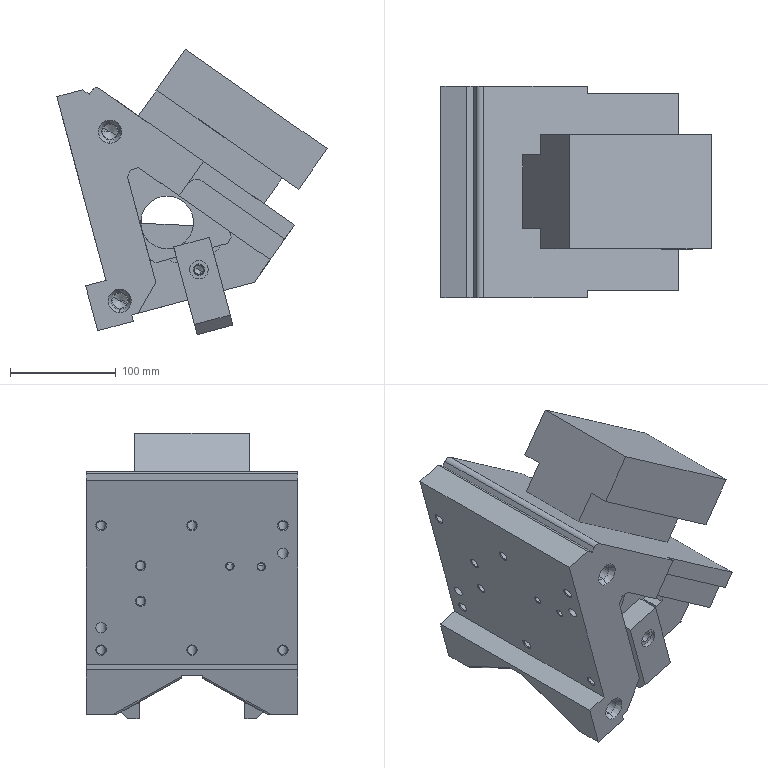Part | NX | features solid 2 | 1 solid | 218 faces | box 255.828 x 200 x 270.136 mm | volume 5105228 mm3 | plane 107 | cylinder 67 | cone 44 | commonest cylinder face diameters 16 x16 14.2 x10 8.5 x8 10 x7 4 x4 8.6 x4